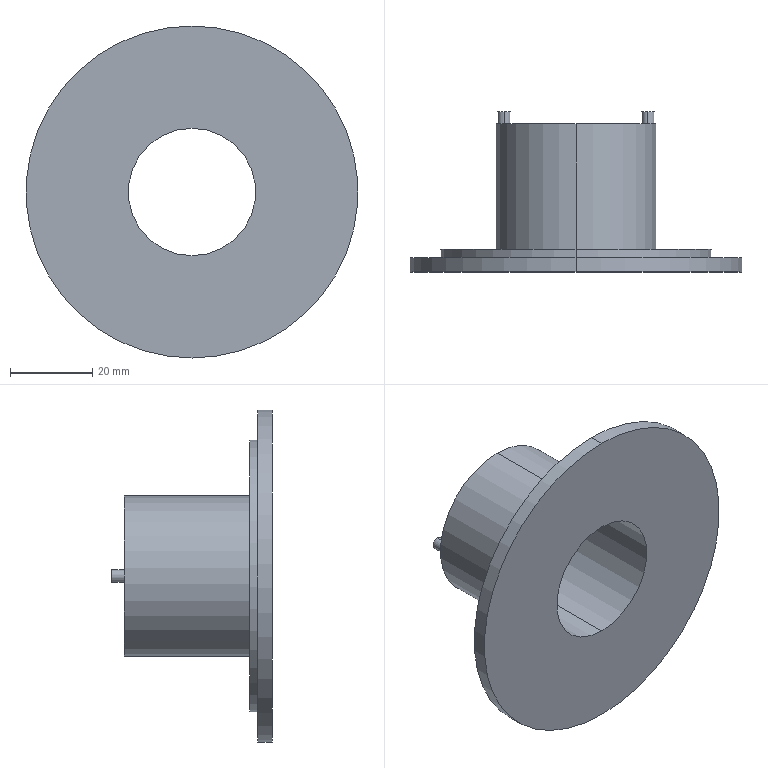Part | SolidWorks | features ICE 1, Revolution 1 | 1 solid | 18 faces | box 80.737 x 39 x 80.737 mm | volume 34067 mm3 | cylinder 12 | plane 6 | commonest cylinder face diameters 3 x4 31 x2 39 x2 66 x2 80.737 x2
STEP:
#1=CARTESIAN_POINT('',(-17.5,176.5,1.5));
#2=VERTEX_POINT('',#1);
#3=CARTESIAN_POINT('',(-17.5,176.5,-1.5));
#4=VERTEX_POINT('',#3);
#5=CARTESIAN_POINT('',(-17.5,176.5,0.));
#6=DIRECTION('',(0.,1.,0.));
#7=DIRECTION('',(0.,0.,1.));
#8=AXIS2_PLACEMENT_3D('',#5,#6,#7);
#9=CIRCLE('',#8,1.5);
#10=EDGE_CURVE('',#2,#4,#9,.T.);
#11=ORIENTED_EDGE('',*,*,#10,.F.);
#12=CARTESIAN_POINT('',(-17.5,173.5,1.5));
#13=VERTEX_POINT('',#12);
#14=CARTESIAN_POINT('',(-17.5,176.5,1.5));
#15=DIRECTION('',(0.,-1.,0.));
#16=VECTOR('',#15,1000.);
#17=LINE('',#14,#16);
#18=EDGE_CURVE('',#2,#13,#17,.T.);
#19=ORIENTED_EDGE('',*,*,#18,.T.);
#20=CARTESIAN_POINT('',(-17.5,173.5,-1.5));
#21=VERTEX_POINT('',#20);
#22=CARTESIAN_POINT('',(-17.5,173.5,0.));
#23=DIRECTION('',(0.,1.,0.));
#24=DIRECTION('',(0.,0.,1.));
#25=AXIS2_PLACEMENT_3D('',#22,#23,#24);
#26=CIRCLE('',#25,1.5);
#27=EDGE_CURVE('',#13,#21,#26,.T.);
#28=ORIENTED_EDGE('',*,*,#27,.T.);
#29=CARTESIAN_POINT('',(-17.5,176.5,-1.5));
#30=DIRECTION('',(0.,-1.,0.));
#31=VECTOR('',#30,1000.);
#32=LINE('',#29,#31);
#33=EDGE_CURVE('',#4,#21,#32,.T.);
#34=ORIENTED_EDGE('',*,*,#33,.F.);
#35=EDGE_LOOP('',(#11,#19,#28,#34));
#36=FACE_OUTER_BOUND('',#35,.T.);
#37=CARTESIAN_POINT('',(-17.5,176.5,0.));
#38=DIRECTION('',(0.,-1.,0.));
#39=DIRECTION('',(0.,0.,-1.));
#40=AXIS2_PLACEMENT_3D('',#37,#38,#39);
#41=CYLINDRICAL_SURFACE('',#40,1.5);
#42=ADVANCED_FACE('',(#36),#41,.T.);
#43=CARTESIAN_POINT('',(17.5,176.5,1.5));
#44=VERTEX_POINT('',#43);
#45=CARTESIAN_POINT('',(17.5,176.5,-1.5));
#46=VERTEX_POINT('',#45);
#47=CARTESIAN_POINT('',(17.5,176.5,0.));
#48=DIRECTION('',(0.,1.,0.));
#49=DIRECTION('',(0.,0.,1.));
#50=AXIS2_PLACEMENT_3D('',#47,#48,#49);
#51=CIRCLE('',#50,1.5);
#52=EDGE_CURVE('',#44,#46,#51,.T.);
#53=ORIENTED_EDGE('',*,*,#52,.F.);
#54=CARTESIAN_POINT('',(17.5,173.5,1.5));
#55=VERTEX_POINT('',#54);
#56=CARTESIAN_POINT('',(17.5,176.5,1.5));
#57=DIRECTION('',(0.,-1.,0.));
#58=VECTOR('',#57,1000.);
#59=LINE('',#56,#58);
#60=EDGE_CURVE('',#44,#55,#59,.T.);
#61=ORIENTED_EDGE('',*,*,#60,.T.);
#62=CARTESIAN_POINT('',(17.5,173.5,-1.5));
#63=VERTEX_POINT('',#62);
#64=CARTESIAN_POINT('',(17.5,173.5,0.));
#65=DIRECTION('',(0.,1.,0.));
#66=DIRECTION('',(0.,0.,1.));
#67=AXIS2_PLACEMENT_3D('',#64,#65,#66);
#68=CIRCLE('',#67,1.5);
#69=EDGE_CURVE('',#55,#63,#68,.T.);
#70=ORIENTED_EDGE('',*,*,#69,.T.);
#71=CARTESIAN_POINT('',(17.5,176.5,-1.5));
#72=DIRECTION('',(0.,-1.,0.));
#73=VECTOR('',#72,1000.);
#74=LINE('',#71,#73);
#75=EDGE_CURVE('',#46,#63,#74,.T.);
#76=ORIENTED_EDGE('',*,*,#75,.F.);
#77=EDGE_LOOP('',(#53,#61,#70,#76));
#78=FACE_OUTER_BOUND('',#77,.T.);
#79=CARTESIAN_POINT('',(17.5,176.5,0.));
#80=DIRECTION('',(0.,-1.,0.));
#81=DIRECTION('',(0.,0.,-1.));
#82=AXIS2_PLACEMENT_3D('',#79,#80,#81);
#83=CYLINDRICAL_SURFACE('',#82,1.5);
#84=ADVANCED_FACE('',(#78),#83,.T.);
#85=CARTESIAN_POINT('',(0.,173.5,15.5));
#86=VERTEX_POINT('',#85);
#87=CARTESIAN_POINT('',(0.,173.5,-15.5));
#88=VERTEX_POINT('',#87);
#89=CARTESIAN_POINT('',(0.,173.5,0.));
#90=DIRECTION('',(0.,-1.,0.));
#91=DIRECTION('',(0.,0.,-1.));
#92=AXIS2_PLACEMENT_3D('',#89,#90,#91);
#93=CIRCLE('',#92,15.5);
#94=EDGE_CURVE('',#86,#88,#93,.T.);
#95=ORIENTED_EDGE('',*,*,#94,.F.);
#96=CARTESIAN_POINT('',(0.,137.5,15.5));
#97=VERTEX_POINT('',#96);
#98=CARTESIAN_POINT('',(0.,0.,15.5));
#99=DIRECTION('',(0.,-1.,0.));
#100=VECTOR('',#99,1000.);
#101=LINE('',#98,#100);
#102=EDGE_CURVE('',#86,#97,#101,.T.);
#103=ORIENTED_EDGE('',*,*,#102,.T.);
#104=CARTESIAN_POINT('',(0.,137.5,-15.5));
#105=VERTEX_POINT('',#104);
#106=CARTESIAN_POINT('',(0.,137.5,0.));
#107=DIRECTION('',(0.,-1.,0.));
#108=DIRECTION('',(0.,0.,-1.));
#109=AXIS2_PLACEMENT_3D('',#106,#107,#108);
#110=CIRCLE('',#109,15.5);
#111=EDGE_CURVE('',#97,#105,#110,.T.);
#112=ORIENTED_EDGE('',*,*,#111,.T.);
#113=CARTESIAN_POINT('',(0.,0.,-15.5));
#114=DIRECTION('',(0.,-1.,0.));
#115=VECTOR('',#114,1000.);
#116=LINE('',#113,#115);
#117=EDGE_CURVE('',#88,#105,#116,.T.);
#118=ORIENTED_EDGE('',*,*,#117,.F.);
#119=EDGE_LOOP('',(#95,#103,#112,#118));
#120=FACE_OUTER_BOUND('',#119,.T.);
#121=CARTESIAN_POINT('',(0.,0.,0.));
#122=DIRECTION('',(0.,-1.,0.));
#123=DIRECTION('',(0.,0.,-1.));
#124=AXIS2_PLACEMENT_3D('',#121,#122,#123);
#125=CYLINDRICAL_SURFACE('',#124,15.5);
#126=ADVANCED_FACE('',(#120),#125,.F.);
#127=CARTESIAN_POINT('',(0.,173.5,-19.5));
#128=VERTEX_POINT('',#127);
#129=CARTESIAN_POINT('',(0.,173.5,19.5));
#130=VERTEX_POINT('',#129);
#131=CARTESIAN_POINT('',(0.,173.5,0.));
#132=DIRECTION('',(0.,-1.,0.));
#133=DIRECTION('',(0.,0.,-1.));
#134=AXIS2_PLACEMENT_3D('',#131,#132,#133);
#135=CIRCLE('',#134,19.5);
#136=EDGE_CURVE('',#128,#130,#135,.T.);
#137=ORIENTED_EDGE('',*,*,#136,.T.);
#138=CARTESIAN_POINT('',(0.,143.,19.5));
#139=VERTEX_POINT('',#138);
#140=CARTESIAN_POINT('',(0.,0.,19.5));
#141=DIRECTION('',(0.,-1.,0.));
#142=VECTOR('',#141,1000.);
#143=LINE('',#140,#142);
#144=EDGE_CURVE('',#130,#139,#143,.T.);
#145=ORIENTED_EDGE('',*,*,#144,.T.);
#146=CARTESIAN_POINT('',(0.,143.,-19.5));
#147=VERTEX_POINT('',#146);
#148=CARTESIAN_POINT('',(0.,143.,0.));
#149=DIRECTION('',(0.,-1.,0.));
#150=DIRECTION('',(0.,0.,-1.));
#151=AXIS2_PLACEMENT_3D('',#148,#149,#150);
#152=CIRCLE('',#151,19.5);
#153=EDGE_CURVE('',#147,#139,#152,.T.);
#154=ORIENTED_EDGE('',*,*,#153,.F.);
#155=CARTESIAN_POINT('',(0.,0.,-19.5));
#156=DIRECTION('',(0.,-1.,0.));
#157=VECTOR('',#156,1000.);
#158=LINE('',#155,#157);
#159=EDGE_CURVE('',#128,#147,#158,.T.);
#160=ORIENTED_EDGE('',*,*,#159,.F.);
#161=EDGE_LOOP('',(#137,#145,#154,#160));
#162=FACE_OUTER_BOUND('',#161,.T.);
#163=CARTESIAN_POINT('',(0.,0.,0.));
#164=DIRECTION('',(0.,-1.,0.));
#165=DIRECTION('',(0.,0.,-1.));
#166=AXIS2_PLACEMENT_3D('',#163,#164,#165);
#167=CYLINDRICAL_SURFACE('',#166,19.5);
#168=ADVANCED_FACE('',(#162),#167,.T.);
#169=CARTESIAN_POINT('',(0.,143.,-33.));
#170=VERTEX_POINT('',#169);
#171=CARTESIAN_POINT('',(0.,143.,33.));
#172=VERTEX_POINT('',#171);
#173=CARTESIAN_POINT('',(0.,143.,0.));
#174=DIRECTION('',(0.,-1.,0.));
#175=DIRECTION('',(0.,0.,-1.));
#176=AXIS2_PLACEMENT_3D('',#173,#174,#175);
#177=CIRCLE('',#176,33.);
#178=EDGE_CURVE('',#170,#172,#177,.T.);
#179=ORIENTED_EDGE('',*,*,#178,.T.);
#180=CARTESIAN_POINT('',(0.,141.,33.));
#181=VERTEX_POINT('',#180);
#182=CARTESIAN_POINT('',(0.,0.,33.));
#183=DIRECTION('',(0.,-1.,0.));
#184=VECTOR('',#183,1000.);
#185=LINE('',#182,#184);
#186=EDGE_CURVE('',#172,#181,#185,.T.);
#187=ORIENTED_EDGE('',*,*,#186,.T.);
#188=CARTESIAN_POINT('',(0.,141.,-33.));
#189=VERTEX_POINT('',#188);
#190=CARTESIAN_POINT('',(0.,141.,0.));
#191=DIRECTION('',(0.,-1.,0.));
#192=DIRECTION('',(0.,0.,-1.));
#193=AXIS2_PLACEMENT_3D('',#190,#191,#192);
#194=CIRCLE('',#193,33.);
#195=EDGE_CURVE('',#189,#181,#194,.T.);
#196=ORIENTED_EDGE('',*,*,#195,.F.);
#197=CARTESIAN_POINT('',(0.,0.,-33.));
#198=DIRECTION('',(0.,-1.,0.));
#199=VECTOR('',#198,1000.);
#200=LINE('',#197,#199);
#201=EDGE_CURVE('',#170,#189,#200,.T.);
#202=ORIENTED_EDGE('',*,*,#201,.F.);
#203=EDGE_LOOP('',(#179,#187,#196,#202));
#204=FACE_OUTER_BOUND('',#203,.T.);
#205=CARTESIAN_POINT('',(0.,0.,0.));
#206=DIRECTION('',(0.,-1.,0.));
#207=DIRECTION('',(0.,0.,-1.));
#208=AXIS2_PLACEMENT_3D('',#205,#206,#207);
#209=CYLINDRICAL_SURFACE('',#208,33.);
#210=ADVANCED_FACE('',(#204),#209,.T.);
#211=CARTESIAN_POINT('',(0.,141.,-40.369));
#212=VERTEX_POINT('',#211);
#213=CARTESIAN_POINT('',(0.,141.,40.369));
#214=VERTEX_POINT('',#213);
#215=CARTESIAN_POINT('',(0.,141.,0.));
#216=DIRECTION('',(0.,-1.,0.));
#217=DIRECTION('',(0.,0.,-1.));
#218=AXIS2_PLACEMENT_3D('',#215,#216,#217);
#219=CIRCLE('',#218,40.369);
#220=EDGE_CURVE('',#212,#214,#219,.T.);
#221=ORIENTED_EDGE('',*,*,#220,.T.);
#222=CARTESIAN_POINT('',(0.,137.5,40.369));
#223=VERTEX_POINT('',#222);
#224=CARTESIAN_POINT('',(0.,0.,40.369));
#225=DIRECTION('',(0.,-1.,0.));
#226=VECTOR('',#225,1000.);
#227=LINE('',#224,#226);
#228=EDGE_CURVE('',#214,#223,#227,.T.);
#229=ORIENTED_EDGE('',*,*,#228,.T.);
#230=CARTESIAN_POINT('',(0.,137.5,-40.369));
#231=VERTEX_POINT('',#230);
#232=CARTESIAN_POINT('',(0.,137.5,0.));
#233=DIRECTION('',(0.,-1.,0.));
#234=DIRECTION('',(0.,0.,-1.));
#235=AXIS2_PLACEMENT_3D('',#232,#233,#234);
#236=CIRCLE('',#235,40.369);
#237=EDGE_CURVE('',#231,#223,#236,.T.);
#238=ORIENTED_EDGE('',*,*,#237,.F.);
#239=CARTESIAN_POINT('',(0.,0.,-40.369));
#240=DIRECTION('',(0.,-1.,0.));
#241=VECTOR('',#240,1000.);
#242=LINE('',#239,#241);
#243=EDGE_CURVE('',#212,#231,#242,.T.);
#244=ORIENTED_EDGE('',*,*,#243,.F.);
#245=EDGE_LOOP('',(#221,#229,#238,#244));
#246=FACE_OUTER_BOUND('',#245,.T.);
#247=CARTESIAN_POINT('',(0.,0.,0.));
#248=DIRECTION('',(0.,-1.,0.));
#249=DIRECTION('',(0.,0.,-1.));
#250=AXIS2_PLACEMENT_3D('',#247,#248,#249);
#251=CYLINDRICAL_SURFACE('',#250,40.369);
#252=ADVANCED_FACE('',(#246),#251,.T.);
#253=ORIENTED_EDGE('',*,*,#228,.F.);
#254=CARTESIAN_POINT('',(0.,141.,0.));
#255=DIRECTION('',(0.,-1.,0.));
#256=DIRECTION('',(0.,0.,-1.));
#257=AXIS2_PLACEMENT_3D('',#254,#255,#256);
#258=CIRCLE('',#257,40.369);
#259=EDGE_CURVE('',#214,#212,#258,.T.);
#260=ORIENTED_EDGE('',*,*,#259,.T.);
#261=ORIENTED_EDGE('',*,*,#243,.T.);
#262=CARTESIAN_POINT('',(0.,137.5,0.));
#263=DIRECTION('',(0.,-1.,0.));
#264=DIRECTION('',(0.,0.,-1.));
#265=AXIS2_PLACEMENT_3D('',#262,#263,#264);
#266=CIRCLE('',#265,40.369);
#267=EDGE_CURVE('',#223,#231,#266,.T.);
#268=ORIENTED_EDGE('',*,*,#267,.F.);
#269=EDGE_LOOP('',(#253,#260,#261,#268));
#270=FACE_OUTER_BOUND('',#269,.T.);
#271=CARTESIAN_POINT('',(0.,0.,0.));
#272=DIRECTION('',(0.,-1.,0.));
#273=DIRECTION('',(0.,0.,-1.));
#274=AXIS2_PLACEMENT_3D('',#271,#272,#273);
#275=CYLINDRICAL_SURFACE('',#274,40.369);
#276=ADVANCED_FACE('',(#270),#275,.T.);
#277=ORIENTED_EDGE('',*,*,#195,.T.);
#278=CARTESIAN_POINT('',(0.,141.,0.));
#279=DIRECTION('',(0.,-1.,0.));
#280=DIRECTION('',(0.,0.,-1.));
#281=AXIS2_PLACEMENT_3D('',#278,#279,#280);
#282=CIRCLE('',#281,33.);
#283=EDGE_CURVE('',#181,#189,#282,.T.);
#284=ORIENTED_EDGE('',*,*,#283,.T.);
#285=EDGE_LOOP('',(#277,#284));
#286=FACE_BOUND('',#285,.T.);
#287=ORIENTED_EDGE('',*,*,#220,.F.);
#288=ORIENTED_EDGE('',*,*,#259,.F.);
#289=EDGE_LOOP('',(#287,#288));
#290=FACE_OUTER_BOUND('',#289,.T.);
#291=CARTESIAN_POINT('',(40.369,141.,0.));
#292=DIRECTION('',(0.,1.,0.));
#293=DIRECTION('',(0.,0.,1.));
#294=AXIS2_PLACEMENT_3D('',#291,#292,#293);
#295=PLANE('',#294);
#296=ADVANCED_FACE('',(#286,#290),#295,.T.);
#297=ORIENTED_EDGE('',*,*,#186,.F.);
#298=CARTESIAN_POINT('',(0.,143.,0.));
#299=DIRECTION('',(0.,-1.,0.));
#300=DIRECTION('',(0.,0.,-1.));
#301=AXIS2_PLACEMENT_3D('',#298,#299,#300);
#302=CIRCLE('',#301,33.);
#303=EDGE_CURVE('',#172,#170,#302,.T.);
#304=ORIENTED_EDGE('',*,*,#303,.T.);
#305=ORIENTED_EDGE('',*,*,#201,.T.);
#306=ORIENTED_EDGE('',*,*,#283,.F.);
#307=EDGE_LOOP('',(#297,#304,#305,#306));
#308=FACE_OUTER_BOUND('',#307,.T.);
#309=CARTESIAN_POINT('',(0.,0.,0.));
#310=DIRECTION('',(0.,-1.,0.));
#311=DIRECTION('',(0.,0.,-1.));
#312=AXIS2_PLACEMENT_3D('',#309,#310,#311);
#313=CYLINDRICAL_SURFACE('',#312,33.);
#314=ADVANCED_FACE('',(#308),#313,.T.);
#315=ORIENTED_EDGE('',*,*,#153,.T.);
#316=CARTESIAN_POINT('',(0.,143.,0.));
#317=DIRECTION('',(0.,-1.,0.));
#318=DIRECTION('',(0.,0.,-1.));
#319=AXIS2_PLACEMENT_3D('',#316,#317,#318);
#320=CIRCLE('',#319,19.5);
#321=EDGE_CURVE('',#139,#147,#320,.T.);
#322=ORIENTED_EDGE('',*,*,#321,.T.);
#323=EDGE_LOOP('',(#315,#322));
#324=FACE_BOUND('',#323,.T.);
#325=ORIENTED_EDGE('',*,*,#178,.F.);
#326=ORIENTED_EDGE('',*,*,#303,.F.);
#327=EDGE_LOOP('',(#325,#326));
#328=FACE_OUTER_BOUND('',#327,.T.);
#329=CARTESIAN_POINT('',(33.,143.,0.));
#330=DIRECTION('',(0.,1.,0.));
#331=DIRECTION('',(0.,0.,1.));
#332=AXIS2_PLACEMENT_3D('',#329,#330,#331);
#333=PLANE('',#332);
#334=ADVANCED_FACE('',(#324,#328),#333,.T.);
#335=ORIENTED_EDGE('',*,*,#144,.F.);
#336=CARTESIAN_POINT('',(0.,173.5,0.));
#337=DIRECTION('',(0.,-1.,0.));
#338=DIRECTION('',(0.,0.,-1.));
#339=AXIS2_PLACEMENT_3D('',#336,#337,#338);
#340=CIRCLE('',#339,19.5);
#341=EDGE_CURVE('',#130,#128,#340,.T.);
#342=ORIENTED_EDGE('',*,*,#341,.T.);
#343=ORIENTED_EDGE('',*,*,#159,.T.);
#344=ORIENTED_EDGE('',*,*,#321,.F.);
#345=EDGE_LOOP('',(#335,#342,#343,#344));
#346=FACE_OUTER_BOUND('',#345,.T.);
#347=CARTESIAN_POINT('',(0.,0.,0.));
#348=DIRECTION('',(0.,-1.,0.));
#349=DIRECTION('',(0.,0.,-1.));
#350=AXIS2_PLACEMENT_3D('',#347,#348,#349);
#351=CYLINDRICAL_SURFACE('',#350,19.5);
#352=ADVANCED_FACE('',(#346),#351,.T.);
#353=CARTESIAN_POINT('',(-17.5,173.5,0.));
#354=DIRECTION('',(0.,1.,0.));
#355=DIRECTION('',(0.,0.,1.));
#356=AXIS2_PLACEMENT_3D('',#353,#354,#355);
#357=CIRCLE('',#356,1.5);
#358=EDGE_CURVE('',#21,#13,#357,.T.);
#359=ORIENTED_EDGE('',*,*,#358,.F.);
#360=ORIENTED_EDGE('',*,*,#27,.F.);
#361=EDGE_LOOP('',(#359,#360));
#362=FACE_BOUND('',#361,.T.);
#363=CARTESIAN_POINT('',(17.5,173.5,0.));
#364=DIRECTION('',(0.,1.,0.));
#365=DIRECTION('',(0.,0.,1.));
#366=AXIS2_PLACEMENT_3D('',#363,#364,#365);
#367=CIRCLE('',#366,1.5);
#368=EDGE_CURVE('',#63,#55,#367,.T.);
#369=ORIENTED_EDGE('',*,*,#368,.F.);
#370=ORIENTED_EDGE('',*,*,#69,.F.);
#371=EDGE_LOOP('',(#369,#370));
#372=FACE_BOUND('',#371,.T.);
#373=CARTESIAN_POINT('',(0.,173.5,0.));
#374=DIRECTION('',(0.,-1.,0.));
#375=DIRECTION('',(0.,0.,-1.));
#376=AXIS2_PLACEMENT_3D('',#373,#374,#375);
#377=CIRCLE('',#376,15.5);
#378=EDGE_CURVE('',#88,#86,#377,.T.);
#379=ORIENTED_EDGE('',*,*,#378,.T.);
#380=ORIENTED_EDGE('',*,*,#94,.T.);
#381=EDGE_LOOP('',(#379,#380));
#382=FACE_BOUND('',#381,.T.);
#383=ORIENTED_EDGE('',*,*,#136,.F.);
#384=ORIENTED_EDGE('',*,*,#341,.F.);
#385=EDGE_LOOP('',(#383,#384));
#386=FACE_OUTER_BOUND('',#385,.T.);
#387=CARTESIAN_POINT('',(19.5,173.5,0.));
#388=DIRECTION('',(0.,1.,0.));
#389=DIRECTION('',(0.,0.,1.));
#390=AXIS2_PLACEMENT_3D('',#387,#388,#389);
#391=PLANE('',#390);
#392=ADVANCED_FACE('',(#362,#372,#382,#386),#391,.T.);
#393=ORIENTED_EDGE('',*,*,#102,.F.);
#394=ORIENTED_EDGE('',*,*,#378,.F.);
#395=ORIENTED_EDGE('',*,*,#117,.T.);
#396=CARTESIAN_POINT('',(0.,137.5,0.));
#397=DIRECTION('',(0.,-1.,0.));
#398=DIRECTION('',(0.,0.,-1.));
#399=AXIS2_PLACEMENT_3D('',#396,#397,#398);
#400=CIRCLE('',#399,15.5);
#401=EDGE_CURVE('',#105,#97,#400,.T.);
#402=ORIENTED_EDGE('',*,*,#401,.T.);
#403=EDGE_LOOP('',(#393,#394,#395,#402));
#404=FACE_OUTER_BOUND('',#403,.T.);
#405=CARTESIAN_POINT('',(0.,0.,0.));
#406=DIRECTION('',(0.,-1.,0.));
#407=DIRECTION('',(0.,0.,-1.));
#408=AXIS2_PLACEMENT_3D('',#405,#406,#407);
#409=CYLINDRICAL_SURFACE('',#408,15.5);
#410=ADVANCED_FACE('',(#404),#409,.F.);
#411=ORIENTED_EDGE('',*,*,#237,.T.);
#412=ORIENTED_EDGE('',*,*,#267,.T.);
#413=EDGE_LOOP('',(#411,#412));
#414=FACE_OUTER_BOUND('',#413,.T.);
#415=ORIENTED_EDGE('',*,*,#401,.F.);
#416=ORIENTED_EDGE('',*,*,#111,.F.);
#417=EDGE_LOOP('',(#415,#416));
#418=FACE_BOUND('',#417,.T.);
#419=CARTESIAN_POINT('',(29.304,137.5,0.));
#420=DIRECTION('',(0.,-1.,0.));
#421=DIRECTION('',(0.,0.,-1.));
#422=AXIS2_PLACEMENT_3D('',#419,#420,#421);
#423=PLANE('',#422);
#424=ADVANCED_FACE('',(#414,#418),#423,.T.);
#425=ORIENTED_EDGE('',*,*,#60,.F.);
#426=CARTESIAN_POINT('',(17.5,176.5,0.));
#427=DIRECTION('',(0.,1.,0.));
#428=DIRECTION('',(0.,0.,1.));
#429=AXIS2_PLACEMENT_3D('',#426,#427,#428);
#430=CIRCLE('',#429,1.5);
#431=EDGE_CURVE('',#46,#44,#430,.T.);
#432=ORIENTED_EDGE('',*,*,#431,.F.);
#433=ORIENTED_EDGE('',*,*,#75,.T.);
#434=ORIENTED_EDGE('',*,*,#368,.T.);
#435=EDGE_LOOP('',(#425,#432,#433,#434));
#436=FACE_OUTER_BOUND('',#435,.T.);
#437=CARTESIAN_POINT('',(17.5,176.5,0.));
#438=DIRECTION('',(0.,-1.,0.));
#439=DIRECTION('',(0.,0.,-1.));
#440=AXIS2_PLACEMENT_3D('',#437,#438,#439);
#441=CYLINDRICAL_SURFACE('',#440,1.5);
#442=ADVANCED_FACE('',(#436),#441,.T.);
#443=ORIENTED_EDGE('',*,*,#431,.T.);
#444=ORIENTED_EDGE('',*,*,#52,.T.);
#445=EDGE_LOOP('',(#443,#444));
#446=FACE_OUTER_BOUND('',#445,.T.);
#447=CARTESIAN_POINT('',(17.5,176.5,0.));
#448=DIRECTION('',(0.,1.,0.));
#449=DIRECTION('',(0.,0.,1.));
#450=AXIS2_PLACEMENT_3D('',#447,#448,#449);
#451=PLANE('',#450);
#452=ADVANCED_FACE('',(#446),#451,.T.);
#453=ORIENTED_EDGE('',*,*,#18,.F.);
#454=CARTESIAN_POINT('',(-17.5,176.5,0.));
#455=DIRECTION('',(0.,1.,0.));
#456=DIRECTION('',(0.,0.,1.));
#457=AXIS2_PLACEMENT_3D('',#454,#455,#456);
#458=CIRCLE('',#457,1.5);
#459=EDGE_CURVE('',#4,#2,#458,.T.);
#460=ORIENTED_EDGE('',*,*,#459,.F.);
#461=ORIENTED_EDGE('',*,*,#33,.T.);
#462=ORIENTED_EDGE('',*,*,#358,.T.);
#463=EDGE_LOOP('',(#453,#460,#461,#462));
#464=FACE_OUTER_BOUND('',#463,.T.);
#465=CARTESIAN_POINT('',(-17.5,176.5,0.));
#466=DIRECTION('',(0.,-1.,0.));
#467=DIRECTION('',(0.,0.,-1.));
#468=AXIS2_PLACEMENT_3D('',#465,#466,#467);
#469=CYLINDRICAL_SURFACE('',#468,1.5);
#470=ADVANCED_FACE('',(#464),#469,.T.);
#471=ORIENTED_EDGE('',*,*,#459,.T.);
#472=ORIENTED_EDGE('',*,*,#10,.T.);
#473=EDGE_LOOP('',(#471,#472));
#474=FACE_OUTER_BOUND('',#473,.T.);
#475=CARTESIAN_POINT('',(-17.5,176.5,0.));
#476=DIRECTION('',(0.,1.,0.));
#477=DIRECTION('',(0.,0.,1.));
#478=AXIS2_PLACEMENT_3D('',#475,#476,#477);
#479=PLANE('',#478);
#480=ADVANCED_FACE('',(#474),#479,.T.);
#481=CLOSED_SHELL('',(#42,#84,#126,#168,#210,#252,#276,#296,#314,#334,#352,#392,#410,#424,#442,#452,#470,#480));
#482=MANIFOLD_SOLID_BREP('',#481);
#483=CARTESIAN_POINT('',(0.,0.,0.));
#484=DIRECTION('',(0.,0.,1.));
#485=DIRECTION('',(1.,0.,0.));
#486=AXIS2_PLACEMENT_3D('',#483,#484,#485);
#487=(LENGTH_UNIT()NAMED_UNIT(*)SI_UNIT(.MILLI.,.METRE.));
#488=UNCERTAINTY_MEASURE_WITH_UNIT(LENGTH_MEASURE(0.00001),#487,'','');
#489=(NAMED_UNIT(*)PLANE_ANGLE_UNIT()SI_UNIT($,.RADIAN.));
#490=(NAMED_UNIT(*)SI_UNIT($,.STERADIAN.)SOLID_ANGLE_UNIT());
#491=(GEOMETRIC_REPRESENTATION_CONTEXT(3)GLOBAL_UNCERTAINTY_ASSIGNED_CONTEXT((#488))GLOBAL_UNIT_ASSIGNED_CONTEXT((#487,#489,#490))REPRESENTATION_CONTEXT('',''));
#492=ADVANCED_BREP_SHAPE_REPRESENTATION('',(#482,#486),#491);